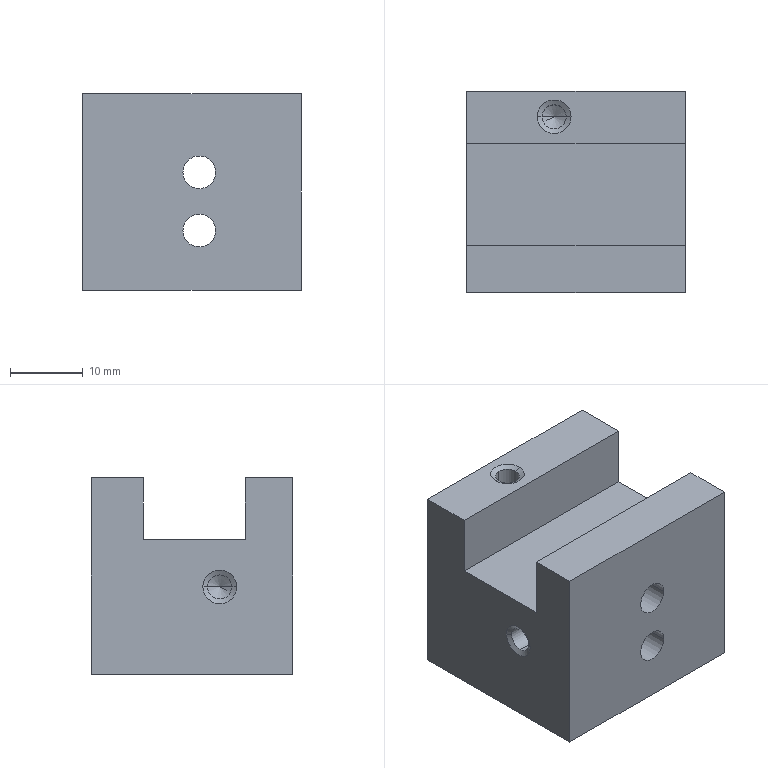Part | NX | 1 solid | 32 faces | box 30 x 27.6 x 27 mm | volume 17582 mm3 | cone 12 | plane 10 | cylinder 10 | commonest cylinder face diameters 3.3 x6 4.5 x4
STEP:
#1=CARTESIAN_POINT('',(30.,6.5,0.));
#2=VERTEX_POINT('',#1);
#3=CARTESIAN_POINT('',(0.,6.5,0.));
#4=VERTEX_POINT('',#3);
#5=CARTESIAN_POINT('',(30.,6.5,0.));
#6=DIRECTION('',(-1.,0.,0.));
#7=VECTOR('',#6,1000.);
#8=LINE('',#5,#7);
#9=EDGE_CURVE('',#2,#4,#8,.T.);
#10=ORIENTED_EDGE('',*,*,#9,.T.);
#11=CARTESIAN_POINT('',(0.,0.,0.));
#12=VERTEX_POINT('',#11);
#13=CARTESIAN_POINT('',(0.,0.,0.));
#14=DIRECTION('',(0.,-1.,0.));
#15=VECTOR('',#14,1000.);
#16=LINE('',#13,#15);
#17=EDGE_CURVE('',#4,#12,#16,.T.);
#18=ORIENTED_EDGE('',*,*,#17,.T.);
#19=CARTESIAN_POINT('',(30.,0.,0.));
#20=VERTEX_POINT('',#19);
#21=CARTESIAN_POINT('',(0.,0.,0.));
#22=DIRECTION('',(1.,0.,0.));
#23=VECTOR('',#22,1000.);
#24=LINE('',#21,#23);
#25=EDGE_CURVE('',#12,#20,#24,.T.);
#26=ORIENTED_EDGE('',*,*,#25,.T.);
#27=CARTESIAN_POINT('',(30.,0.,0.));
#28=DIRECTION('',(0.,1.,0.));
#29=VECTOR('',#28,1000.);
#30=LINE('',#27,#29);
#31=EDGE_CURVE('',#20,#2,#30,.T.);
#32=ORIENTED_EDGE('',*,*,#31,.T.);
#33=EDGE_LOOP('',(#10,#18,#26,#32));
#34=FACE_BOUND('',#33,.T.);
#35=CARTESIAN_POINT('',(0.,0.,0.));
#36=DIRECTION('',(0.,0.,1.));
#37=DIRECTION('',(1.,0.,0.));
#38=AXIS2_PLACEMENT_3D('',#35,#36,#37);
#39=PLANE('',#38);
#40=ADVANCED_FACE('',(#34),#39,.T.);
#41=ORIENTED_EDGE('',*,*,#9,.F.);
#42=CARTESIAN_POINT('',(30.,6.5,-8.5));
#43=VERTEX_POINT('',#42);
#44=CARTESIAN_POINT('',(30.,6.5,-8.5));
#45=DIRECTION('',(0.,0.,1.));
#46=VECTOR('',#45,1000.);
#47=LINE('',#44,#46);
#48=EDGE_CURVE('',#43,#2,#47,.T.);
#49=ORIENTED_EDGE('',*,*,#48,.F.);
#50=CARTESIAN_POINT('',(0.,6.5,-8.5));
#51=VERTEX_POINT('',#50);
#52=CARTESIAN_POINT('',(0.,6.5,-8.5));
#53=DIRECTION('',(1.,0.,0.));
#54=VECTOR('',#53,1000.);
#55=LINE('',#52,#54);
#56=EDGE_CURVE('',#51,#43,#55,.T.);
#57=ORIENTED_EDGE('',*,*,#56,.F.);
#58=CARTESIAN_POINT('',(0.,6.5,0.));
#59=DIRECTION('',(0.,0.,-1.));
#60=VECTOR('',#59,1000.);
#61=LINE('',#58,#60);
#62=EDGE_CURVE('',#4,#51,#61,.T.);
#63=ORIENTED_EDGE('',*,*,#62,.F.);
#64=EDGE_LOOP('',(#41,#49,#57,#63));
#65=FACE_BOUND('',#64,.T.);
#66=CARTESIAN_POINT('',(30.,6.5,0.));
#67=DIRECTION('',(0.,-1.,0.));
#68=DIRECTION('',(0.,0.,-1.));
#69=AXIS2_PLACEMENT_3D('',#66,#67,#68);
#70=PLANE('',#69);
#71=ADVANCED_FACE('',(#65),#70,.F.);
#72=ORIENTED_EDGE('',*,*,#62,.T.);
#73=CARTESIAN_POINT('',(0.,20.5,-8.5));
#74=VERTEX_POINT('',#73);
#75=CARTESIAN_POINT('',(0.,0.,-8.5));
#76=DIRECTION('',(0.,1.,0.));
#77=VECTOR('',#76,1000.);
#78=LINE('',#75,#77);
#79=EDGE_CURVE('',#51,#74,#78,.T.);
#80=ORIENTED_EDGE('',*,*,#79,.T.);
#81=CARTESIAN_POINT('',(0.,20.5,0.));
#82=VERTEX_POINT('',#81);
#83=CARTESIAN_POINT('',(0.,20.5,0.));
#84=DIRECTION('',(0.,0.,1.));
#85=VECTOR('',#84,1000.);
#86=LINE('',#83,#85);
#87=EDGE_CURVE('',#74,#82,#86,.T.);
#88=ORIENTED_EDGE('',*,*,#87,.T.);
#89=CARTESIAN_POINT('',(0.,27.6,0.));
#90=VERTEX_POINT('',#89);
#91=CARTESIAN_POINT('',(0.,0.,0.));
#92=DIRECTION('',(0.,1.,0.));
#93=VECTOR('',#92,1000.);
#94=LINE('',#91,#93);
#95=EDGE_CURVE('',#82,#90,#94,.T.);
#96=ORIENTED_EDGE('',*,*,#95,.T.);
#97=CARTESIAN_POINT('',(0.,27.6,-27.));
#98=VERTEX_POINT('',#97);
#99=CARTESIAN_POINT('',(0.,27.6,0.));
#100=DIRECTION('',(0.,0.,1.));
#101=VECTOR('',#100,1000.);
#102=LINE('',#99,#101);
#103=EDGE_CURVE('',#98,#90,#102,.T.);
#104=ORIENTED_EDGE('',*,*,#103,.F.);
#105=CARTESIAN_POINT('',(0.,0.,-27.));
#106=VERTEX_POINT('',#105);
#107=CARTESIAN_POINT('',(0.,0.,-27.));
#108=DIRECTION('',(0.,-1.,0.));
#109=VECTOR('',#108,1000.);
#110=LINE('',#107,#109);
#111=EDGE_CURVE('',#98,#106,#110,.T.);
#112=ORIENTED_EDGE('',*,*,#111,.T.);
#113=CARTESIAN_POINT('',(0.,0.,0.));
#114=DIRECTION('',(0.,0.,-1.));
#115=VECTOR('',#114,1000.);
#116=LINE('',#113,#115);
#117=EDGE_CURVE('',#12,#106,#116,.T.);
#118=ORIENTED_EDGE('',*,*,#117,.F.);
#119=ORIENTED_EDGE('',*,*,#17,.F.);
#120=EDGE_LOOP('',(#72,#80,#88,#96,#104,#112,#118,#119));
#121=FACE_BOUND('',#120,.T.);
#122=CARTESIAN_POINT('',(0.,7.685,-15.));
#123=VERTEX_POINT('',#122);
#124=CARTESIAN_POINT('',(0.,12.315,-15.));
#125=VERTEX_POINT('',#124);
#126=CARTESIAN_POINT('',(0.,10.,-15.));
#127=DIRECTION('',(-1.,0.,0.));
#128=DIRECTION('',(0.,1.,0.));
#129=AXIS2_PLACEMENT_3D('',#126,#127,#128);
#130=CIRCLE('',#129,2.315);
#131=EDGE_CURVE('',#123,#125,#130,.T.);
#132=ORIENTED_EDGE('',*,*,#131,.F.);
#133=CARTESIAN_POINT('',(0.,10.,-15.));
#134=DIRECTION('',(-1.,0.,0.));
#135=DIRECTION('',(0.,1.,0.));
#136=AXIS2_PLACEMENT_3D('',#133,#134,#135);
#137=CIRCLE('',#136,2.315);
#138=EDGE_CURVE('',#125,#123,#137,.T.);
#139=ORIENTED_EDGE('',*,*,#138,.F.);
#140=EDGE_LOOP('',(#132,#139));
#141=FACE_BOUND('',#140,.T.);
#142=CARTESIAN_POINT('',(0.,27.6,0.));
#143=DIRECTION('',(-1.,0.,0.));
#144=DIRECTION('',(0.,0.,1.));
#145=AXIS2_PLACEMENT_3D('',#142,#143,#144);
#146=PLANE('',#145);
#147=ADVANCED_FACE('',(#121,#141),#146,.T.);
#148=ORIENTED_EDGE('',*,*,#25,.F.);
#149=ORIENTED_EDGE('',*,*,#117,.T.);
#150=CARTESIAN_POINT('',(30.,0.,-27.));
#151=VERTEX_POINT('',#150);
#152=CARTESIAN_POINT('',(0.,0.,-27.));
#153=DIRECTION('',(-1.,0.,0.));
#154=VECTOR('',#153,1000.);
#155=LINE('',#152,#154);
#156=EDGE_CURVE('',#151,#106,#155,.T.);
#157=ORIENTED_EDGE('',*,*,#156,.F.);
#158=CARTESIAN_POINT('',(30.,0.,0.));
#159=DIRECTION('',(0.,0.,-1.));
#160=VECTOR('',#159,1000.);
#161=LINE('',#158,#160);
#162=EDGE_CURVE('',#20,#151,#161,.T.);
#163=ORIENTED_EDGE('',*,*,#162,.F.);
#164=EDGE_LOOP('',(#148,#149,#157,#163));
#165=FACE_BOUND('',#164,.T.);
#166=CARTESIAN_POINT('',(13.75,0.,-18.8));
#167=VERTEX_POINT('',#166);
#168=CARTESIAN_POINT('',(18.25,0.,-18.8));
#169=VERTEX_POINT('',#168);
#170=CARTESIAN_POINT('',(16.,0.,-18.8));
#171=DIRECTION('',(0.,-1.,0.));
#172=DIRECTION('',(-1.,0.,0.));
#173=AXIS2_PLACEMENT_3D('',#170,#171,#172);
#174=CIRCLE('',#173,2.25);
#175=EDGE_CURVE('',#167,#169,#174,.T.);
#176=ORIENTED_EDGE('',*,*,#175,.F.);
#177=CARTESIAN_POINT('',(16.,0.,-18.8));
#178=DIRECTION('',(0.,-1.,0.));
#179=DIRECTION('',(-1.,0.,0.));
#180=AXIS2_PLACEMENT_3D('',#177,#178,#179);
#181=CIRCLE('',#180,2.25);
#182=EDGE_CURVE('',#169,#167,#181,.T.);
#183=ORIENTED_EDGE('',*,*,#182,.F.);
#184=EDGE_LOOP('',(#176,#183));
#185=FACE_BOUND('',#184,.T.);
#186=CARTESIAN_POINT('',(18.25,0.,-10.8));
#187=VERTEX_POINT('',#186);
#188=CARTESIAN_POINT('',(13.75,0.,-10.8));
#189=VERTEX_POINT('',#188);
#190=CARTESIAN_POINT('',(16.,0.,-10.8));
#191=DIRECTION('',(0.,-1.,0.));
#192=DIRECTION('',(-1.,0.,0.));
#193=AXIS2_PLACEMENT_3D('',#190,#191,#192);
#194=CIRCLE('',#193,2.25);
#195=EDGE_CURVE('',#187,#189,#194,.T.);
#196=ORIENTED_EDGE('',*,*,#195,.F.);
#197=CARTESIAN_POINT('',(16.,0.,-10.8));
#198=DIRECTION('',(0.,-1.,0.));
#199=DIRECTION('',(-1.,0.,0.));
#200=AXIS2_PLACEMENT_3D('',#197,#198,#199);
#201=CIRCLE('',#200,2.25);
#202=EDGE_CURVE('',#189,#187,#201,.T.);
#203=ORIENTED_EDGE('',*,*,#202,.F.);
#204=EDGE_LOOP('',(#196,#203));
#205=FACE_BOUND('',#204,.T.);
#206=CARTESIAN_POINT('',(0.,0.,0.));
#207=DIRECTION('',(0.,-1.,0.));
#208=DIRECTION('',(0.,0.,-1.));
#209=AXIS2_PLACEMENT_3D('',#206,#207,#208);
#210=PLANE('',#209);
#211=ADVANCED_FACE('',(#165,#185,#205),#210,.T.);
#212=ORIENTED_EDGE('',*,*,#48,.T.);
#213=ORIENTED_EDGE('',*,*,#31,.F.);
#214=ORIENTED_EDGE('',*,*,#162,.T.);
#215=CARTESIAN_POINT('',(30.,27.6,-27.));
#216=VERTEX_POINT('',#215);
#217=CARTESIAN_POINT('',(30.,0.,-27.));
#218=DIRECTION('',(0.,-1.,0.));
#219=VECTOR('',#218,1000.);
#220=LINE('',#217,#219);
#221=EDGE_CURVE('',#216,#151,#220,.T.);
#222=ORIENTED_EDGE('',*,*,#221,.F.);
#223=CARTESIAN_POINT('',(30.,27.6,0.));
#224=VERTEX_POINT('',#223);
#225=CARTESIAN_POINT('',(30.,27.6,0.));
#226=DIRECTION('',(0.,0.,-1.));
#227=VECTOR('',#226,1000.);
#228=LINE('',#225,#227);
#229=EDGE_CURVE('',#224,#216,#228,.T.);
#230=ORIENTED_EDGE('',*,*,#229,.F.);
#231=CARTESIAN_POINT('',(30.,20.5,0.));
#232=VERTEX_POINT('',#231);
#233=CARTESIAN_POINT('',(30.,0.,0.));
#234=DIRECTION('',(0.,-1.,0.));
#235=VECTOR('',#234,1000.);
#236=LINE('',#233,#235);
#237=EDGE_CURVE('',#224,#232,#236,.T.);
#238=ORIENTED_EDGE('',*,*,#237,.T.);
#239=CARTESIAN_POINT('',(30.,20.5,-8.5));
#240=VERTEX_POINT('',#239);
#241=CARTESIAN_POINT('',(30.,20.5,-8.5));
#242=DIRECTION('',(0.,0.,1.));
#243=VECTOR('',#242,1000.);
#244=LINE('',#241,#243);
#245=EDGE_CURVE('',#240,#232,#244,.T.);
#246=ORIENTED_EDGE('',*,*,#245,.F.);
#247=CARTESIAN_POINT('',(30.,20.5,-8.5));
#248=DIRECTION('',(0.,-1.,0.));
#249=VECTOR('',#248,1000.);
#250=LINE('',#247,#249);
#251=EDGE_CURVE('',#240,#43,#250,.T.);
#252=ORIENTED_EDGE('',*,*,#251,.T.);
#253=EDGE_LOOP('',(#212,#213,#214,#222,#230,#238,#246,#252));
#254=FACE_BOUND('',#253,.T.);
#255=CARTESIAN_POINT('',(30.,0.,0.));
#256=DIRECTION('',(1.,0.,0.));
#257=DIRECTION('',(0.,1.,0.));
#258=AXIS2_PLACEMENT_3D('',#255,#256,#257);
#259=PLANE('',#258);
#260=ADVANCED_FACE('',(#254),#259,.T.);
#261=ORIENTED_EDGE('',*,*,#251,.F.);
#262=CARTESIAN_POINT('',(0.,20.5,-8.5));
#263=DIRECTION('',(1.,0.,0.));
#264=VECTOR('',#263,1000.);
#265=LINE('',#262,#264);
#266=EDGE_CURVE('',#74,#240,#265,.T.);
#267=ORIENTED_EDGE('',*,*,#266,.F.);
#268=ORIENTED_EDGE('',*,*,#79,.F.);
#269=ORIENTED_EDGE('',*,*,#56,.T.);
#270=EDGE_LOOP('',(#261,#267,#268,#269));
#271=FACE_BOUND('',#270,.T.);
#272=CARTESIAN_POINT('',(30.,6.5,-8.5));
#273=DIRECTION('',(0.,0.,-1.));
#274=DIRECTION('',(0.,-1.,0.));
#275=AXIS2_PLACEMENT_3D('',#272,#273,#274);
#276=PLANE('',#275);
#277=ADVANCED_FACE('',(#271),#276,.F.);
#278=CARTESIAN_POINT('',(0.,20.5,0.));
#279=DIRECTION('',(1.,0.,0.));
#280=VECTOR('',#279,1000.);
#281=LINE('',#278,#280);
#282=EDGE_CURVE('',#82,#232,#281,.T.);
#283=ORIENTED_EDGE('',*,*,#282,.F.);
#284=ORIENTED_EDGE('',*,*,#87,.F.);
#285=ORIENTED_EDGE('',*,*,#266,.T.);
#286=ORIENTED_EDGE('',*,*,#245,.T.);
#287=EDGE_LOOP('',(#283,#284,#285,#286));
#288=FACE_BOUND('',#287,.T.);
#289=CARTESIAN_POINT('',(30.,20.5,-8.5));
#290=DIRECTION('',(0.,1.,0.));
#291=DIRECTION('',(1.,0.,0.));
#292=AXIS2_PLACEMENT_3D('',#289,#290,#291);
#293=PLANE('',#292);
#294=ADVANCED_FACE('',(#288),#293,.F.);
#295=ORIENTED_EDGE('',*,*,#282,.T.);
#296=ORIENTED_EDGE('',*,*,#237,.F.);
#297=CARTESIAN_POINT('',(0.,27.6,0.));
#298=DIRECTION('',(1.,0.,0.));
#299=VECTOR('',#298,1000.);
#300=LINE('',#297,#299);
#301=EDGE_CURVE('',#90,#224,#300,.T.);
#302=ORIENTED_EDGE('',*,*,#301,.F.);
#303=ORIENTED_EDGE('',*,*,#95,.F.);
#304=EDGE_LOOP('',(#295,#296,#302,#303));
#305=FACE_BOUND('',#304,.T.);
#306=CARTESIAN_POINT('',(14.315,24.1,0.));
#307=VERTEX_POINT('',#306);
#308=CARTESIAN_POINT('',(9.685,24.1,0.));
#309=VERTEX_POINT('',#308);
#310=CARTESIAN_POINT('',(12.,24.1,0.));
#311=DIRECTION('',(0.,0.,1.));
#312=DIRECTION('',(1.,0.,0.));
#313=AXIS2_PLACEMENT_3D('',#310,#311,#312);
#314=CIRCLE('',#313,2.315);
#315=EDGE_CURVE('',#307,#309,#314,.T.);
#316=ORIENTED_EDGE('',*,*,#315,.F.);
#317=CARTESIAN_POINT('',(12.,24.1,0.));
#318=DIRECTION('',(0.,0.,1.));
#319=DIRECTION('',(1.,0.,0.));
#320=AXIS2_PLACEMENT_3D('',#317,#318,#319);
#321=CIRCLE('',#320,2.315);
#322=EDGE_CURVE('',#309,#307,#321,.T.);
#323=ORIENTED_EDGE('',*,*,#322,.F.);
#324=EDGE_LOOP('',(#316,#323));
#325=FACE_BOUND('',#324,.T.);
#326=CARTESIAN_POINT('',(0.,0.,0.));
#327=DIRECTION('',(0.,0.,1.));
#328=DIRECTION('',(1.,0.,0.));
#329=AXIS2_PLACEMENT_3D('',#326,#327,#328);
#330=PLANE('',#329);
#331=ADVANCED_FACE('',(#305,#325),#330,.T.);
#332=ORIENTED_EDGE('',*,*,#301,.T.);
#333=ORIENTED_EDGE('',*,*,#229,.T.);
#334=CARTESIAN_POINT('',(0.,27.6,-27.));
#335=DIRECTION('',(1.,0.,0.));
#336=VECTOR('',#335,1000.);
#337=LINE('',#334,#336);
#338=EDGE_CURVE('',#98,#216,#337,.T.);
#339=ORIENTED_EDGE('',*,*,#338,.F.);
#340=ORIENTED_EDGE('',*,*,#103,.T.);
#341=EDGE_LOOP('',(#332,#333,#339,#340));
#342=FACE_BOUND('',#341,.T.);
#343=CARTESIAN_POINT('',(13.75,27.6,-18.8));
#344=VERTEX_POINT('',#343);
#345=CARTESIAN_POINT('',(18.25,27.6,-18.8));
#346=VERTEX_POINT('',#345);
#347=CARTESIAN_POINT('',(16.,27.6,-18.8));
#348=DIRECTION('',(0.,1.,0.));
#349=DIRECTION('',(1.,0.,0.));
#350=AXIS2_PLACEMENT_3D('',#347,#348,#349);
#351=CIRCLE('',#350,2.25);
#352=EDGE_CURVE('',#344,#346,#351,.T.);
#353=ORIENTED_EDGE('',*,*,#352,.F.);
#354=CARTESIAN_POINT('',(16.,27.6,-18.8));
#355=DIRECTION('',(0.,1.,0.));
#356=DIRECTION('',(1.,0.,0.));
#357=AXIS2_PLACEMENT_3D('',#354,#355,#356);
#358=CIRCLE('',#357,2.25);
#359=EDGE_CURVE('',#346,#344,#358,.T.);
#360=ORIENTED_EDGE('',*,*,#359,.F.);
#361=EDGE_LOOP('',(#353,#360));
#362=FACE_BOUND('',#361,.T.);
#363=CARTESIAN_POINT('',(18.25,27.6,-10.8));
#364=VERTEX_POINT('',#363);
#365=CARTESIAN_POINT('',(13.75,27.6,-10.8));
#366=VERTEX_POINT('',#365);
#367=CARTESIAN_POINT('',(16.,27.6,-10.8));
#368=DIRECTION('',(0.,1.,0.));
#369=DIRECTION('',(1.,0.,0.));
#370=AXIS2_PLACEMENT_3D('',#367,#368,#369);
#371=CIRCLE('',#370,2.25);
#372=EDGE_CURVE('',#364,#366,#371,.T.);
#373=ORIENTED_EDGE('',*,*,#372,.F.);
#374=CARTESIAN_POINT('',(16.,27.6,-10.8));
#375=DIRECTION('',(0.,1.,0.));
#376=DIRECTION('',(1.,0.,0.));
#377=AXIS2_PLACEMENT_3D('',#374,#375,#376);
#378=CIRCLE('',#377,2.25);
#379=EDGE_CURVE('',#366,#364,#378,.T.);
#380=ORIENTED_EDGE('',*,*,#379,.F.);
#381=EDGE_LOOP('',(#373,#380));
#382=FACE_BOUND('',#381,.T.);
#383=CARTESIAN_POINT('',(30.,27.6,0.));
#384=DIRECTION('',(0.,1.,0.));
#385=DIRECTION('',(1.,0.,0.));
#386=AXIS2_PLACEMENT_3D('',#383,#384,#385);
#387=PLANE('',#386);
#388=ADVANCED_FACE('',(#342,#362,#382),#387,.T.);
#389=ORIENTED_EDGE('',*,*,#156,.T.);
#390=ORIENTED_EDGE('',*,*,#111,.F.);
#391=ORIENTED_EDGE('',*,*,#338,.T.);
#392=ORIENTED_EDGE('',*,*,#221,.T.);
#393=EDGE_LOOP('',(#389,#390,#391,#392));
#394=FACE_BOUND('',#393,.T.);
#395=CARTESIAN_POINT('',(19.685,15.6,-27.));
#396=VERTEX_POINT('',#395);
#397=CARTESIAN_POINT('',(24.315,15.6,-27.));
#398=VERTEX_POINT('',#397);
#399=CARTESIAN_POINT('',(22.,15.6,-27.));
#400=DIRECTION('',(0.,0.,-1.));
#401=DIRECTION('',(-1.,0.,0.));
#402=AXIS2_PLACEMENT_3D('',#399,#400,#401);
#403=CIRCLE('',#402,2.315);
#404=EDGE_CURVE('',#396,#398,#403,.T.);
#405=ORIENTED_EDGE('',*,*,#404,.F.);
#406=CARTESIAN_POINT('',(22.,15.6,-27.));
#407=DIRECTION('',(0.,0.,-1.));
#408=DIRECTION('',(-1.,0.,0.));
#409=AXIS2_PLACEMENT_3D('',#406,#407,#408);
#410=CIRCLE('',#409,2.315);
#411=EDGE_CURVE('',#398,#396,#410,.T.);
#412=ORIENTED_EDGE('',*,*,#411,.F.);
#413=EDGE_LOOP('',(#405,#412));
#414=FACE_BOUND('',#413,.T.);
#415=CARTESIAN_POINT('',(0.,0.,-27.));
#416=DIRECTION('',(0.,0.,1.));
#417=DIRECTION('',(1.,0.,0.));
#418=AXIS2_PLACEMENT_3D('',#415,#416,#417);
#419=PLANE('',#418);
#420=ADVANCED_FACE('',(#394,#414),#419,.F.);
#421=ORIENTED_EDGE('',*,*,#372,.T.);
#422=CARTESIAN_POINT('',(13.75,27.6,-10.8));
#423=DIRECTION('',(0.,-1.,0.));
#424=VECTOR('',#423,1000.);
#425=LINE('',#422,#424);
#426=EDGE_CURVE('',#189,#366,#425,.F.);
#427=ORIENTED_EDGE('',*,*,#426,.F.);
#428=ORIENTED_EDGE('',*,*,#202,.T.);
#429=CARTESIAN_POINT('',(18.25,27.6,-10.8));
#430=DIRECTION('',(0.,-1.,0.));
#431=VECTOR('',#430,1000.);
#432=LINE('',#429,#431);
#433=EDGE_CURVE('',#187,#364,#432,.F.);
#434=ORIENTED_EDGE('',*,*,#433,.T.);
#435=EDGE_LOOP('',(#421,#427,#428,#434));
#436=FACE_BOUND('',#435,.T.);
#437=CARTESIAN_POINT('',(16.,27.6,-10.8));
#438=DIRECTION('',(0.,-1.,0.));
#439=DIRECTION('',(1.,0.,0.));
#440=AXIS2_PLACEMENT_3D('',#437,#438,#439);
#441=CYLINDRICAL_SURFACE('',#440,2.25);
#442=ADVANCED_FACE('',(#436),#441,.F.);
#443=CARTESIAN_POINT('',(22.,15.6,-13.809));
#444=VERTEX_POINT('',#443);
#445=CARTESIAN_POINT('',(23.65,15.6,-14.8));
#446=VERTEX_POINT('',#445);
#447=CARTESIAN_POINT('',(23.65,15.6,-14.8));
#448=DIRECTION('',(0.8572,0.,-0.515));
#449=VECTOR('',#448,1000.);
#450=LINE('',#447,#449);
#451=EDGE_CURVE('',#444,#446,#450,.T.);
#452=ORIENTED_EDGE('',*,*,#451,.T.);
#453=CARTESIAN_POINT('',(22.,13.95,-14.8));
#454=VERTEX_POINT('',#453);
#455=CARTESIAN_POINT('',(22.,15.6,-14.8));
#456=DIRECTION('',(0.,0.,1.));
#457=DIRECTION('',(1.,0.,0.));
#458=AXIS2_PLACEMENT_3D('',#455,#456,#457);
#459=CIRCLE('',#458,1.65);
#460=EDGE_CURVE('',#454,#446,#459,.T.);
#461=ORIENTED_EDGE('',*,*,#460,.F.);
#462=CARTESIAN_POINT('',(20.35,15.6,-14.8));
#463=VERTEX_POINT('',#462);
#464=CARTESIAN_POINT('',(22.,15.6,-14.8));
#465=DIRECTION('',(0.,0.,1.));
#466=DIRECTION('',(1.,0.,0.));
#467=AXIS2_PLACEMENT_3D('',#464,#465,#466);
#468=CIRCLE('',#467,1.65);
#469=EDGE_CURVE('',#463,#454,#468,.T.);
#470=ORIENTED_EDGE('',*,*,#469,.F.);
#471=CARTESIAN_POINT('',(20.35,15.6,-14.8));
#472=DIRECTION('',(-0.8572,0.,-0.515));
#473=VECTOR('',#472,1000.);
#474=LINE('',#471,#473);
#475=EDGE_CURVE('',#444,#463,#474,.T.);
#476=ORIENTED_EDGE('',*,*,#475,.F.);
#477=EDGE_LOOP('',(#452,#461,#470,#476));
#478=FACE_BOUND('',#477,.T.);
#479=CARTESIAN_POINT('',(22.,15.6,-14.8));
#480=DIRECTION('',(0.,0.,-1.));
#481=DIRECTION('',(-1.,0.,0.));
#482=AXIS2_PLACEMENT_3D('',#479,#480,#481);
#483=CONICAL_SURFACE('',#482,1.65,1.03);
#484=ADVANCED_FACE('',(#478),#483,.F.);
#485=CARTESIAN_POINT('',(12.2,11.65,-15.));
#486=VERTEX_POINT('',#485);
#487=CARTESIAN_POINT('',(12.2,10.,-13.35));
#488=VERTEX_POINT('',#487);
#489=CARTESIAN_POINT('',(12.2,10.,-15.));
#490=DIRECTION('',(1.,0.,0.));
#491=DIRECTION('',(0.,1.,0.));
#492=AXIS2_PLACEMENT_3D('',#489,#490,#491);
#493=CIRCLE('',#492,1.65);
#494=EDGE_CURVE('',#486,#488,#493,.T.);
#495=ORIENTED_EDGE('',*,*,#494,.T.);
#496=CARTESIAN_POINT('',(0.3839,10.,-13.35));
#497=VERTEX_POINT('',#496);
#498=CARTESIAN_POINT('',(10.1,10.,-13.35));
#499=DIRECTION('',(-1.,0.,0.));
#500=VECTOR('',#499,1000.);
#501=LINE('',#498,#500);
#502=EDGE_CURVE('',#497,#488,#501,.F.);
#503=ORIENTED_EDGE('',*,*,#502,.F.);
#504=CARTESIAN_POINT('',(0.3839,11.65,-15.));
#505=VERTEX_POINT('',#504);
#506=CARTESIAN_POINT('',(0.3839,10.,-15.));
#507=DIRECTION('',(-1.,0.,0.));
#508=DIRECTION('',(0.,1.,0.));
#509=AXIS2_PLACEMENT_3D('',#506,#507,#508);
#510=CIRCLE('',#509,1.65);
#511=EDGE_CURVE('',#497,#505,#510,.T.);
#512=ORIENTED_EDGE('',*,*,#511,.T.);
#513=CARTESIAN_POINT('',(0.3839,10.,-16.65));
#514=VERTEX_POINT('',#513);
#515=CARTESIAN_POINT('',(0.3839,10.,-15.));
#516=DIRECTION('',(-1.,0.,0.));
#517=DIRECTION('',(0.,1.,0.));
#518=AXIS2_PLACEMENT_3D('',#515,#516,#517);
#519=CIRCLE('',#518,1.65);
#520=EDGE_CURVE('',#505,#514,#519,.T.);
#521=ORIENTED_EDGE('',*,*,#520,.T.);
#522=CARTESIAN_POINT('',(12.2,10.,-16.65));
#523=VERTEX_POINT('',#522);
#524=CARTESIAN_POINT('',(10.1,10.,-16.65));
#525=DIRECTION('',(-1.,0.,0.));
#526=VECTOR('',#525,1000.);
#527=LINE('',#524,#526);
#528=EDGE_CURVE('',#514,#523,#527,.F.);
#529=ORIENTED_EDGE('',*,*,#528,.T.);
#530=CARTESIAN_POINT('',(12.2,10.,-15.));
#531=DIRECTION('',(1.,0.,0.));
#532=DIRECTION('',(0.,1.,0.));
#533=AXIS2_PLACEMENT_3D('',#530,#531,#532);
#534=CIRCLE('',#533,1.65);
#535=EDGE_CURVE('',#523,#486,#534,.T.);
#536=ORIENTED_EDGE('',*,*,#535,.T.);
#537=EDGE_LOOP('',(#495,#503,#512,#521,#529,#536));
#538=FACE_BOUND('',#537,.T.);
#539=CARTESIAN_POINT('',(10.1,10.,-15.));
#540=DIRECTION('',(-1.,0.,0.));
#541=DIRECTION('',(0.,0.,1.));
#542=AXIS2_PLACEMENT_3D('',#539,#540,#541);
#543=CYLINDRICAL_SURFACE('',#542,1.65);
#544=ADVANCED_FACE('',(#538),#543,.F.);
#545=ORIENTED_EDGE('',*,*,#315,.T.);
#546=CARTESIAN_POINT('',(10.35,24.1,-0.3839));
#547=VERTEX_POINT('',#546);
#548=CARTESIAN_POINT('',(10.35,24.1,-0.3839));
#549=DIRECTION('',(-0.866,0.,0.5));
#550=VECTOR('',#549,1000.);
#551=LINE('',#548,#550);
#552=EDGE_CURVE('',#547,#309,#551,.T.);
#553=ORIENTED_EDGE('',*,*,#552,.F.);
#554=CARTESIAN_POINT('',(12.,25.75,-0.3839));
#555=VERTEX_POINT('',#554);
#556=CARTESIAN_POINT('',(12.,24.1,-0.3839));
#557=DIRECTION('',(0.,0.,1.));
#558=DIRECTION('',(1.,0.,0.));
#559=AXIS2_PLACEMENT_3D('',#556,#557,#558);
#560=CIRCLE('',#559,1.65);
#561=EDGE_CURVE('',#555,#547,#560,.T.);
#562=ORIENTED_EDGE('',*,*,#561,.F.);
#563=CARTESIAN_POINT('',(13.65,24.1,-0.3839));
#564=VERTEX_POINT('',#563);
#565=CARTESIAN_POINT('',(12.,24.1,-0.3839));
#566=DIRECTION('',(0.,0.,1.));
#567=DIRECTION('',(1.,0.,0.));
#568=AXIS2_PLACEMENT_3D('',#565,#566,#567);
#569=CIRCLE('',#568,1.65);
#570=EDGE_CURVE('',#564,#555,#569,.T.);
#571=ORIENTED_EDGE('',*,*,#570,.F.);
#572=CARTESIAN_POINT('',(13.65,24.1,-0.3839));
#573=DIRECTION('',(0.866,0.,0.5));
#574=VECTOR('',#573,1000.);
#575=LINE('',#572,#574);
#576=EDGE_CURVE('',#564,#307,#575,.T.);
#577=ORIENTED_EDGE('',*,*,#576,.T.);
#578=EDGE_LOOP('',(#545,#553,#562,#571,#577));
#579=FACE_BOUND('',#578,.T.);
#580=CARTESIAN_POINT('',(12.,24.1,-0.3839));
#581=DIRECTION('',(0.,0.,1.));
#582=DIRECTION('',(1.,0.,0.));
#583=AXIS2_PLACEMENT_3D('',#580,#581,#582);
#584=CONICAL_SURFACE('',#583,1.65,1.047);
#585=ADVANCED_FACE('',(#579),#584,.F.);
#586=ORIENTED_EDGE('',*,*,#175,.T.);
#587=CARTESIAN_POINT('',(18.25,27.6,-18.8));
#588=DIRECTION('',(0.,-1.,0.));
#589=VECTOR('',#588,1000.);
#590=LINE('',#587,#589);
#591=EDGE_CURVE('',#346,#169,#590,.T.);
#592=ORIENTED_EDGE('',*,*,#591,.F.);
#593=ORIENTED_EDGE('',*,*,#359,.T.);
#594=CARTESIAN_POINT('',(13.75,27.6,-18.8));
#595=DIRECTION('',(0.,-1.,0.));
#596=VECTOR('',#595,1000.);
#597=LINE('',#594,#596);
#598=EDGE_CURVE('',#344,#167,#597,.T.);
#599=ORIENTED_EDGE('',*,*,#598,.T.);
#600=EDGE_LOOP('',(#586,#592,#593,#599));
#601=FACE_BOUND('',#600,.T.);
#602=CARTESIAN_POINT('',(16.,27.6,-18.8));
#603=DIRECTION('',(0.,-1.,0.));
#604=DIRECTION('',(1.,0.,0.));
#605=AXIS2_PLACEMENT_3D('',#602,#603,#604);
#606=CYLINDRICAL_SURFACE('',#605,2.25);
#607=ADVANCED_FACE('',(#601),#606,.F.);
#608=ORIENTED_EDGE('',*,*,#494,.F.);
#609=CARTESIAN_POINT('',(13.191,10.,-15.));
#610=VERTEX_POINT('',#609);
#611=CARTESIAN_POINT('',(12.2,11.65,-15.));
#612=DIRECTION('',(-0.515,0.8572,0.));
#613=VECTOR('',#612,1000.);
#614=LINE('',#611,#613);
#615=EDGE_CURVE('',#486,#610,#614,.F.);
#616=ORIENTED_EDGE('',*,*,#615,.T.);
#617=CARTESIAN_POINT('',(12.2,8.35,-15.));
#618=VERTEX_POINT('',#617);
#619=CARTESIAN_POINT('',(12.2,8.35,-15.));
#620=DIRECTION('',(-0.515,-0.8572,0.));
#621=VECTOR('',#620,1000.);
#622=LINE('',#619,#621);
#623=EDGE_CURVE('',#618,#610,#622,.F.);
#624=ORIENTED_EDGE('',*,*,#623,.F.);
#625=CARTESIAN_POINT('',(12.2,10.,-15.));
#626=DIRECTION('',(1.,0.,0.));
#627=DIRECTION('',(0.,1.,0.));
#628=AXIS2_PLACEMENT_3D('',#625,#626,#627);
#629=CIRCLE('',#628,1.65);
#630=EDGE_CURVE('',#488,#618,#629,.T.);
#631=ORIENTED_EDGE('',*,*,#630,.F.);
#632=EDGE_LOOP('',(#608,#616,#624,#631));
#633=FACE_BOUND('',#632,.T.);
#634=CARTESIAN_POINT('',(12.2,10.,-15.));
#635=DIRECTION('',(-1.,0.,0.));
#636=DIRECTION('',(0.,1.,0.));
#637=AXIS2_PLACEMENT_3D('',#634,#635,#636);
#638=CONICAL_SURFACE('',#637,1.65,1.03);
#639=ADVANCED_FACE('',(#633),#638,.F.);
#640=CARTESIAN_POINT('',(22.,17.25,-14.8));
#641=VERTEX_POINT('',#640);
#642=CARTESIAN_POINT('',(22.,15.6,-14.8));
#643=DIRECTION('',(0.,0.,1.));
#644=DIRECTION('',(1.,0.,0.));
#645=AXIS2_PLACEMENT_3D('',#642,#643,#644);
#646=CIRCLE('',#645,1.65);
#647=EDGE_CURVE('',#446,#641,#646,.T.);
#648=ORIENTED_EDGE('',*,*,#647,.T.);
#649=CARTESIAN_POINT('',(22.,17.25,-26.616));
#650=VERTEX_POINT('',#649);
#651=CARTESIAN_POINT('',(22.,17.25,-23.));
#652=DIRECTION('',(0.,0.,-1.));
#653=VECTOR('',#652,1000.);
#654=LINE('',#651,#653);
#655=EDGE_CURVE('',#641,#650,#654,.T.);
#656=ORIENTED_EDGE('',*,*,#655,.T.);
#657=CARTESIAN_POINT('',(23.65,15.6,-26.616));
#658=VERTEX_POINT('',#657);
#659=CARTESIAN_POINT('',(22.,15.6,-26.616));
#660=DIRECTION('',(0.,0.,-1.));
#661=DIRECTION('',(-1.,0.,0.));
#662=AXIS2_PLACEMENT_3D('',#659,#660,#661);
#663=CIRCLE('',#662,1.65);
#664=EDGE_CURVE('',#650,#658,#663,.T.);
#665=ORIENTED_EDGE('',*,*,#664,.T.);
#666=CARTESIAN_POINT('',(22.,13.95,-26.616));
#667=VERTEX_POINT('',#666);
#668=CARTESIAN_POINT('',(22.,15.6,-26.616));
#669=DIRECTION('',(0.,0.,-1.));
#670=DIRECTION('',(-1.,0.,0.));
#671=AXIS2_PLACEMENT_3D('',#668,#669,#670);
#672=CIRCLE('',#671,1.65);
#673=EDGE_CURVE('',#658,#667,#672,.T.);
#674=ORIENTED_EDGE('',*,*,#673,.T.);
#675=CARTESIAN_POINT('',(22.,13.95,-23.));
#676=DIRECTION('',(0.,0.,-1.));
#677=VECTOR('',#676,1000.);
#678=LINE('',#675,#677);
#679=EDGE_CURVE('',#454,#667,#678,.T.);
#680=ORIENTED_EDGE('',*,*,#679,.F.);
#681=ORIENTED_EDGE('',*,*,#460,.T.);
#682=EDGE_LOOP('',(#648,#656,#665,#674,#680,#681));
#683=FACE_BOUND('',#682,.T.);
#684=CARTESIAN_POINT('',(22.,15.6,-23.));
#685=DIRECTION('',(0.,0.,-1.));
#686=DIRECTION('',(0.,1.,0.));
#687=AXIS2_PLACEMENT_3D('',#684,#685,#686);
#688=CYLINDRICAL_SURFACE('',#687,1.65);
#689=ADVANCED_FACE('',(#683),#688,.F.);
#690=ORIENTED_EDGE('',*,*,#404,.T.);
#691=CARTESIAN_POINT('',(23.65,15.6,-26.616));
#692=DIRECTION('',(0.866,0.,-0.5));
#693=VECTOR('',#692,1000.);
#694=LINE('',#691,#693);
#695=EDGE_CURVE('',#398,#658,#694,.F.);
#696=ORIENTED_EDGE('',*,*,#695,.T.);
#697=ORIENTED_EDGE('',*,*,#664,.F.);
#698=CARTESIAN_POINT('',(20.35,15.6,-26.616));
#699=VERTEX_POINT('',#698);
#700=CARTESIAN_POINT('',(22.,15.6,-26.616));
#701=DIRECTION('',(0.,0.,-1.));
#702=DIRECTION('',(-1.,0.,0.));
#703=AXIS2_PLACEMENT_3D('',#700,#701,#702);
#704=CIRCLE('',#703,1.65);
#705=EDGE_CURVE('',#699,#650,#704,.T.);
#706=ORIENTED_EDGE('',*,*,#705,.F.);
#707=CARTESIAN_POINT('',(20.35,15.6,-26.616));
#708=DIRECTION('',(-0.866,0.,-0.5));
#709=VECTOR('',#708,1000.);
#710=LINE('',#707,#709);
#711=EDGE_CURVE('',#396,#699,#710,.F.);
#712=ORIENTED_EDGE('',*,*,#711,.F.);
#713=EDGE_LOOP('',(#690,#696,#697,#706,#712));
#714=FACE_BOUND('',#713,.T.);
#715=CARTESIAN_POINT('',(22.,15.6,-26.616));
#716=DIRECTION('',(0.,0.,-1.));
#717=DIRECTION('',(-1.,0.,0.));
#718=AXIS2_PLACEMENT_3D('',#715,#716,#717);
#719=CONICAL_SURFACE('',#718,1.65,1.047);
#720=ADVANCED_FACE('',(#714),#719,.F.);
#721=CARTESIAN_POINT('',(12.,25.75,-12.2));
#722=VERTEX_POINT('',#721);
#723=CARTESIAN_POINT('',(13.65,24.1,-12.2));
#724=VERTEX_POINT('',#723);
#725=CARTESIAN_POINT('',(12.,24.1,-12.2));
#726=DIRECTION('',(0.,0.,-1.));
#727=DIRECTION('',(1.,0.,0.));
#728=AXIS2_PLACEMENT_3D('',#725,#726,#727);
#729=CIRCLE('',#728,1.65);
#730=EDGE_CURVE('',#722,#724,#729,.T.);
#731=ORIENTED_EDGE('',*,*,#730,.F.);
#732=CARTESIAN_POINT('',(10.35,24.1,-12.2));
#733=VERTEX_POINT('',#732);
#734=CARTESIAN_POINT('',(12.,24.1,-12.2));
#735=DIRECTION('',(0.,0.,-1.));
#736=DIRECTION('',(1.,0.,0.));
#737=AXIS2_PLACEMENT_3D('',#734,#735,#736);
#738=CIRCLE('',#737,1.65);
#739=EDGE_CURVE('',#733,#722,#738,.T.);
#740=ORIENTED_EDGE('',*,*,#739,.F.);
#741=CARTESIAN_POINT('',(12.,24.1,-13.191));
#742=VERTEX_POINT('',#741);
#743=CARTESIAN_POINT('',(10.35,24.1,-12.2));
#744=DIRECTION('',(-0.8572,0.,0.515));
#745=VECTOR('',#744,1000.);
#746=LINE('',#743,#745);
#747=EDGE_CURVE('',#733,#742,#746,.F.);
#748=ORIENTED_EDGE('',*,*,#747,.T.);
#749=CARTESIAN_POINT('',(13.65,24.1,-12.2));
#750=DIRECTION('',(0.8572,0.,0.515));
#751=VECTOR('',#750,1000.);
#752=LINE('',#749,#751);
#753=EDGE_CURVE('',#724,#742,#752,.F.);
#754=ORIENTED_EDGE('',*,*,#753,.F.);
#755=EDGE_LOOP('',(#731,#740,#748,#754));
#756=FACE_BOUND('',#755,.T.);
#757=CARTESIAN_POINT('',(12.,24.1,-12.2));
#758=DIRECTION('',(0.,0.,1.));
#759=DIRECTION('',(1.,0.,0.));
#760=AXIS2_PLACEMENT_3D('',#757,#758,#759);
#761=CONICAL_SURFACE('',#760,1.65,1.03);
#762=ADVANCED_FACE('',(#756),#761,.F.);
#763=ORIENTED_EDGE('',*,*,#520,.F.);
#764=CARTESIAN_POINT('',(0.3839,11.65,-15.));
#765=DIRECTION('',(-0.5,0.866,0.));
#766=VECTOR('',#765,1000.);
#767=LINE('',#764,#766);
#768=EDGE_CURVE('',#505,#125,#767,.T.);
#769=ORIENTED_EDGE('',*,*,#768,.T.);
#770=ORIENTED_EDGE('',*,*,#138,.T.);
#771=CARTESIAN_POINT('',(0.3839,8.35,-15.));
#772=VERTEX_POINT('',#771);
#773=CARTESIAN_POINT('',(0.3839,8.35,-15.));
#774=DIRECTION('',(-0.5,-0.866,0.));
#775=VECTOR('',#774,1000.);
#776=LINE('',#773,#775);
#777=EDGE_CURVE('',#772,#123,#776,.T.);
#778=ORIENTED_EDGE('',*,*,#777,.F.);
#779=CARTESIAN_POINT('',(0.3839,10.,-15.));
#780=DIRECTION('',(-1.,0.,0.));
#781=DIRECTION('',(0.,1.,0.));
#782=AXIS2_PLACEMENT_3D('',#779,#780,#781);
#783=CIRCLE('',#782,1.65);
#784=EDGE_CURVE('',#514,#772,#783,.T.);
#785=ORIENTED_EDGE('',*,*,#784,.F.);
#786=EDGE_LOOP('',(#763,#769,#770,#778,#785));
#787=FACE_BOUND('',#786,.T.);
#788=CARTESIAN_POINT('',(0.3839,10.,-15.));
#789=DIRECTION('',(-1.,0.,0.));
#790=DIRECTION('',(0.,1.,0.));
#791=AXIS2_PLACEMENT_3D('',#788,#789,#790);
#792=CONICAL_SURFACE('',#791,1.65,1.047);
#793=ADVANCED_FACE('',(#787),#792,.F.);
#794=ORIENTED_EDGE('',*,*,#730,.T.);
#795=CARTESIAN_POINT('',(12.,22.45,-12.2));
#796=VERTEX_POINT('',#795);
#797=CARTESIAN_POINT('',(12.,24.1,-12.2));
#798=DIRECTION('',(0.,0.,-1.));
#799=DIRECTION('',(1.,0.,0.));
#800=AXIS2_PLACEMENT_3D('',#797,#798,#799);
#801=CIRCLE('',#800,1.65);
#802=EDGE_CURVE('',#724,#796,#801,.T.);
#803=ORIENTED_EDGE('',*,*,#802,.T.);
#804=CARTESIAN_POINT('',(12.,22.45,-0.3839));
#805=VERTEX_POINT('',#804);
#806=CARTESIAN_POINT('',(12.,22.45,-4.));
#807=DIRECTION('',(0.,0.,1.));
#808=VECTOR('',#807,1000.);
#809=LINE('',#806,#808);
#810=EDGE_CURVE('',#805,#796,#809,.F.);
#811=ORIENTED_EDGE('',*,*,#810,.F.);
#812=CARTESIAN_POINT('',(12.,24.1,-0.3839));
#813=DIRECTION('',(0.,0.,1.));
#814=DIRECTION('',(1.,0.,0.));
#815=AXIS2_PLACEMENT_3D('',#812,#813,#814);
#816=CIRCLE('',#815,1.65);
#817=EDGE_CURVE('',#805,#564,#816,.T.);
#818=ORIENTED_EDGE('',*,*,#817,.T.);
#819=ORIENTED_EDGE('',*,*,#570,.T.);
#820=CARTESIAN_POINT('',(12.,25.75,-4.));
#821=DIRECTION('',(0.,0.,1.));
#822=VECTOR('',#821,1000.);
#823=LINE('',#820,#822);
#824=EDGE_CURVE('',#555,#722,#823,.F.);
#825=ORIENTED_EDGE('',*,*,#824,.T.);
#826=EDGE_LOOP('',(#794,#803,#811,#818,#819,#825));
#827=FACE_BOUND('',#826,.T.);
#828=CARTESIAN_POINT('',(12.,24.1,-4.));
#829=DIRECTION('',(0.,0.,1.));
#830=DIRECTION('',(0.,-1.,0.));
#831=AXIS2_PLACEMENT_3D('',#828,#829,#830);
#832=CYLINDRICAL_SURFACE('',#831,1.65);
#833=ADVANCED_FACE('',(#827),#832,.F.);
#834=ORIENTED_EDGE('',*,*,#623,.T.);
#835=ORIENTED_EDGE('',*,*,#615,.F.);
#836=ORIENTED_EDGE('',*,*,#535,.F.);
#837=CARTESIAN_POINT('',(12.2,10.,-15.));
#838=DIRECTION('',(1.,0.,0.));
#839=DIRECTION('',(0.,1.,0.));
#840=AXIS2_PLACEMENT_3D('',#837,#838,#839);
#841=CIRCLE('',#840,1.65);
#842=EDGE_CURVE('',#618,#523,#841,.T.);
#843=ORIENTED_EDGE('',*,*,#842,.F.);
#844=EDGE_LOOP('',(#834,#835,#836,#843));
#845=FACE_BOUND('',#844,.T.);
#846=CARTESIAN_POINT('',(12.2,10.,-15.));
#847=DIRECTION('',(-1.,0.,0.));
#848=DIRECTION('',(0.,1.,0.));
#849=AXIS2_PLACEMENT_3D('',#846,#847,#848);
#850=CONICAL_SURFACE('',#849,1.65,1.03);
#851=ADVANCED_FACE('',(#845),#850,.F.);
#852=ORIENTED_EDGE('',*,*,#711,.T.);
#853=CARTESIAN_POINT('',(22.,15.6,-26.616));
#854=DIRECTION('',(0.,0.,-1.));
#855=DIRECTION('',(-1.,0.,0.));
#856=AXIS2_PLACEMENT_3D('',#853,#854,#855);
#857=CIRCLE('',#856,1.65);
#858=EDGE_CURVE('',#667,#699,#857,.T.);
#859=ORIENTED_EDGE('',*,*,#858,.F.);
#860=ORIENTED_EDGE('',*,*,#673,.F.);
#861=ORIENTED_EDGE('',*,*,#695,.F.);
#862=ORIENTED_EDGE('',*,*,#411,.T.);
#863=EDGE_LOOP('',(#852,#859,#860,#861,#862));
#864=FACE_BOUND('',#863,.T.);
#865=CARTESIAN_POINT('',(22.,15.6,-26.616));
#866=DIRECTION('',(0.,0.,-1.));
#867=DIRECTION('',(-1.,0.,0.));
#868=AXIS2_PLACEMENT_3D('',#865,#866,#867);
#869=CONICAL_SURFACE('',#868,1.65,1.047);
#870=ADVANCED_FACE('',(#864),#869,.F.);
#871=ORIENTED_EDGE('',*,*,#747,.F.);
#872=CARTESIAN_POINT('',(12.,24.1,-12.2));
#873=DIRECTION('',(0.,0.,-1.));
#874=DIRECTION('',(1.,0.,0.));
#875=AXIS2_PLACEMENT_3D('',#872,#873,#874);
#876=CIRCLE('',#875,1.65);
#877=EDGE_CURVE('',#796,#733,#876,.T.);
#878=ORIENTED_EDGE('',*,*,#877,.F.);
#879=ORIENTED_EDGE('',*,*,#802,.F.);
#880=ORIENTED_EDGE('',*,*,#753,.T.);
#881=EDGE_LOOP('',(#871,#878,#879,#880));
#882=FACE_BOUND('',#881,.T.);
#883=CARTESIAN_POINT('',(12.,24.1,-12.2));
#884=DIRECTION('',(0.,0.,1.));
#885=DIRECTION('',(1.,0.,0.));
#886=AXIS2_PLACEMENT_3D('',#883,#884,#885);
#887=CONICAL_SURFACE('',#886,1.65,1.03);
#888=ADVANCED_FACE('',(#882),#887,.F.);
#889=ORIENTED_EDGE('',*,*,#131,.T.);
#890=ORIENTED_EDGE('',*,*,#768,.F.);
#891=ORIENTED_EDGE('',*,*,#511,.F.);
#892=CARTESIAN_POINT('',(0.3839,10.,-15.));
#893=DIRECTION('',(-1.,0.,0.));
#894=DIRECTION('',(0.,1.,0.));
#895=AXIS2_PLACEMENT_3D('',#892,#893,#894);
#896=CIRCLE('',#895,1.65);
#897=EDGE_CURVE('',#772,#497,#896,.T.);
#898=ORIENTED_EDGE('',*,*,#897,.F.);
#899=ORIENTED_EDGE('',*,*,#777,.T.);
#900=EDGE_LOOP('',(#889,#890,#891,#898,#899));
#901=FACE_BOUND('',#900,.T.);
#902=CARTESIAN_POINT('',(0.3839,10.,-15.));
#903=DIRECTION('',(-1.,0.,0.));
#904=DIRECTION('',(0.,1.,0.));
#905=AXIS2_PLACEMENT_3D('',#902,#903,#904);
#906=CONICAL_SURFACE('',#905,1.65,1.047);
#907=ADVANCED_FACE('',(#901),#906,.F.);
#908=ORIENTED_EDGE('',*,*,#705,.T.);
#909=ORIENTED_EDGE('',*,*,#655,.F.);
#910=CARTESIAN_POINT('',(22.,15.6,-14.8));
#911=DIRECTION('',(0.,0.,1.));
#912=DIRECTION('',(1.,0.,0.));
#913=AXIS2_PLACEMENT_3D('',#910,#911,#912);
#914=CIRCLE('',#913,1.65);
#915=EDGE_CURVE('',#641,#463,#914,.T.);
#916=ORIENTED_EDGE('',*,*,#915,.T.);
#917=ORIENTED_EDGE('',*,*,#469,.T.);
#918=ORIENTED_EDGE('',*,*,#679,.T.);
#919=ORIENTED_EDGE('',*,*,#858,.T.);
#920=EDGE_LOOP('',(#908,#909,#916,#917,#918,#919));
#921=FACE_BOUND('',#920,.T.);
#922=CARTESIAN_POINT('',(22.,15.6,-23.));
#923=DIRECTION('',(0.,0.,-1.));
#924=DIRECTION('',(0.,1.,0.));
#925=AXIS2_PLACEMENT_3D('',#922,#923,#924);
#926=CYLINDRICAL_SURFACE('',#925,1.65);
#927=ADVANCED_FACE('',(#921),#926,.F.);
#928=ORIENTED_EDGE('',*,*,#352,.T.);
#929=ORIENTED_EDGE('',*,*,#591,.T.);
#930=ORIENTED_EDGE('',*,*,#182,.T.);
#931=ORIENTED_EDGE('',*,*,#598,.F.);
#932=EDGE_LOOP('',(#928,#929,#930,#931));
#933=FACE_BOUND('',#932,.T.);
#934=CARTESIAN_POINT('',(16.,27.6,-18.8));
#935=DIRECTION('',(0.,-1.,0.));
#936=DIRECTION('',(1.,0.,0.));
#937=AXIS2_PLACEMENT_3D('',#934,#935,#936);
#938=CYLINDRICAL_SURFACE('',#937,2.25);
#939=ADVANCED_FACE('',(#933),#938,.F.);
#940=ORIENTED_EDGE('',*,*,#576,.F.);
#941=ORIENTED_EDGE('',*,*,#817,.F.);
#942=CARTESIAN_POINT('',(12.,24.1,-0.3839));
#943=DIRECTION('',(0.,0.,1.));
#944=DIRECTION('',(1.,0.,0.));
#945=AXIS2_PLACEMENT_3D('',#942,#943,#944);
#946=CIRCLE('',#945,1.65);
#947=EDGE_CURVE('',#547,#805,#946,.T.);
#948=ORIENTED_EDGE('',*,*,#947,.F.);
#949=ORIENTED_EDGE('',*,*,#552,.T.);
#950=ORIENTED_EDGE('',*,*,#322,.T.);
#951=EDGE_LOOP('',(#940,#941,#948,#949,#950));
#952=FACE_BOUND('',#951,.T.);
#953=CARTESIAN_POINT('',(12.,24.1,-0.3839));
#954=DIRECTION('',(0.,0.,1.));
#955=DIRECTION('',(1.,0.,0.));
#956=AXIS2_PLACEMENT_3D('',#953,#954,#955);
#957=CONICAL_SURFACE('',#956,1.65,1.047);
#958=ADVANCED_FACE('',(#952),#957,.F.);
#959=ORIENTED_EDGE('',*,*,#528,.F.);
#960=ORIENTED_EDGE('',*,*,#784,.T.);
#961=ORIENTED_EDGE('',*,*,#897,.T.);
#962=ORIENTED_EDGE('',*,*,#502,.T.);
#963=ORIENTED_EDGE('',*,*,#630,.T.);
#964=ORIENTED_EDGE('',*,*,#842,.T.);
#965=EDGE_LOOP('',(#959,#960,#961,#962,#963,#964));
#966=FACE_BOUND('',#965,.T.);
#967=CARTESIAN_POINT('',(10.1,10.,-15.));
#968=DIRECTION('',(-1.,0.,0.));
#969=DIRECTION('',(0.,0.,1.));
#970=AXIS2_PLACEMENT_3D('',#967,#968,#969);
#971=CYLINDRICAL_SURFACE('',#970,1.65);
#972=ADVANCED_FACE('',(#966),#971,.F.);
#973=ORIENTED_EDGE('',*,*,#647,.F.);
#974=ORIENTED_EDGE('',*,*,#451,.F.);
#975=ORIENTED_EDGE('',*,*,#475,.T.);
#976=ORIENTED_EDGE('',*,*,#915,.F.);
#977=EDGE_LOOP('',(#973,#974,#975,#976));
#978=FACE_BOUND('',#977,.T.);
#979=CARTESIAN_POINT('',(22.,15.6,-14.8));
#980=DIRECTION('',(0.,0.,-1.));
#981=DIRECTION('',(-1.,0.,0.));
#982=AXIS2_PLACEMENT_3D('',#979,#980,#981);
#983=CONICAL_SURFACE('',#982,1.65,1.03);
#984=ADVANCED_FACE('',(#978),#983,.F.);
#985=ORIENTED_EDGE('',*,*,#195,.T.);
#986=ORIENTED_EDGE('',*,*,#426,.T.);
#987=ORIENTED_EDGE('',*,*,#379,.T.);
#988=ORIENTED_EDGE('',*,*,#433,.F.);
#989=EDGE_LOOP('',(#985,#986,#987,#988));
#990=FACE_BOUND('',#989,.T.);
#991=CARTESIAN_POINT('',(16.,27.6,-10.8));
#992=DIRECTION('',(0.,-1.,0.));
#993=DIRECTION('',(1.,0.,0.));
#994=AXIS2_PLACEMENT_3D('',#991,#992,#993);
#995=CYLINDRICAL_SURFACE('',#994,2.25);
#996=ADVANCED_FACE('',(#990),#995,.F.);
#997=ORIENTED_EDGE('',*,*,#561,.T.);
#998=ORIENTED_EDGE('',*,*,#947,.T.);
#999=ORIENTED_EDGE('',*,*,#810,.T.);
#1000=ORIENTED_EDGE('',*,*,#877,.T.);
#1001=ORIENTED_EDGE('',*,*,#739,.T.);
#1002=ORIENTED_EDGE('',*,*,#824,.F.);
#1003=EDGE_LOOP('',(#997,#998,#999,#1000,#1001,#1002));
#1004=FACE_BOUND('',#1003,.T.);
#1005=CARTESIAN_POINT('',(12.,24.1,-4.));
#1006=DIRECTION('',(0.,0.,1.));
#1007=DIRECTION('',(0.,-1.,0.));
#1008=AXIS2_PLACEMENT_3D('',#1005,#1006,#1007);
#1009=CYLINDRICAL_SURFACE('',#1008,1.65);
#1010=ADVANCED_FACE('',(#1004),#1009,.F.);
#1011=CLOSED_SHELL('',(#40,#71,#147,#211,#260,#277,#294,#331,#388,#420,#442,#484,#544,#585,#607,#639,#689,#720,#762,#793,#833,#851,#870,#888,#907,#927,#939,#958,#972,#984,#996,#1010));
#1012=MANIFOLD_SOLID_BREP('',#1011);
#1013=(LENGTH_UNIT()NAMED_UNIT(*)SI_UNIT(.MILLI.,.METRE.));
#1014=UNCERTAINTY_MEASURE_WITH_UNIT(LENGTH_MEASURE(0.00001),#1013,'','');
#1015=(NAMED_UNIT(*)PLANE_ANGLE_UNIT()SI_UNIT($,.RADIAN.));
#1016=(NAMED_UNIT(*)SI_UNIT($,.STERADIAN.)SOLID_ANGLE_UNIT());
#1017=(GEOMETRIC_REPRESENTATION_CONTEXT(3)GLOBAL_UNCERTAINTY_ASSIGNED_CONTEXT((#1014))GLOBAL_UNIT_ASSIGNED_CONTEXT((#1013,#1015,#1016))REPRESENTATION_CONTEXT('',''));
#1018=ADVANCED_BREP_SHAPE_REPRESENTATION('',(#1012),#1017);